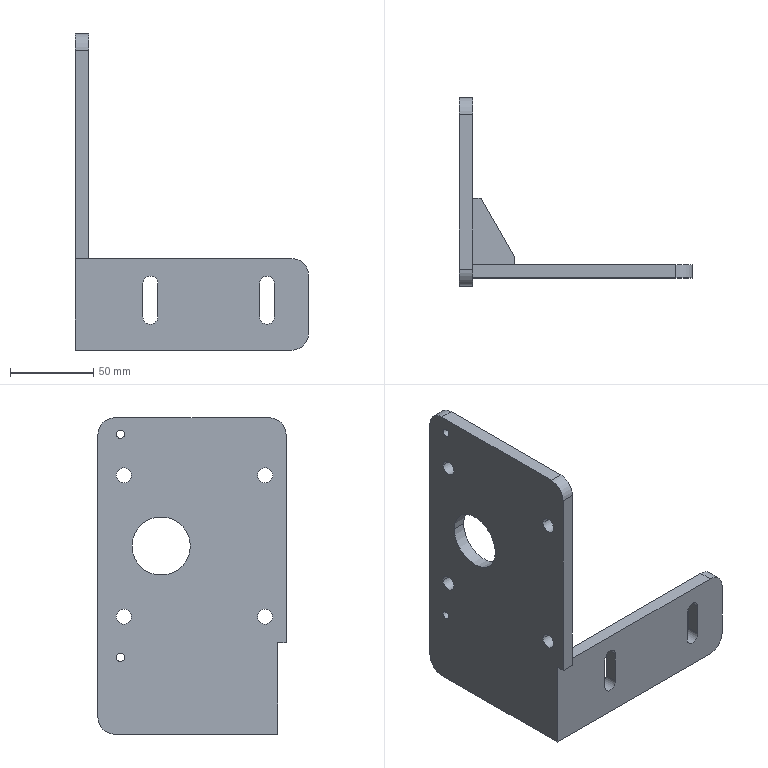Part | SolidWorks | features ICE 6, Fillet 3, Cut 1, DeleteBody 1, ExtruThin 1, MirrorSolid 1 | 2 solids | 47 faces | box 140 x 113 x 190 mm | volume 218037 mm3 | cylinder 25 | plane 22 | commonest cylinder face diameters 9 x14 20 x5 5 x4 35 x2
STEP:
#1=CARTESIAN_POINT('',(8.,48.,-95.));
#2=VERTEX_POINT('',#1);
#3=CARTESIAN_POINT('',(8.,8.,-95.));
#4=VERTEX_POINT('',#3);
#5=CARTESIAN_POINT('',(8.,8.,-95.));
#6=DIRECTION('',(0.,-1.,0.));
#7=VECTOR('',#6,1000.);
#8=LINE('',#5,#7);
#9=EDGE_CURVE('',#2,#4,#8,.T.);
#10=ORIENTED_EDGE('',*,*,#9,.T.);
#11=CARTESIAN_POINT('',(8.,8.,-87.));
#12=VERTEX_POINT('',#11);
#13=CARTESIAN_POINT('',(8.,8.,-87.));
#14=DIRECTION('',(0.,0.,-1.));
#15=VECTOR('',#14,1000.);
#16=LINE('',#13,#15);
#17=EDGE_CURVE('',#12,#4,#16,.T.);
#18=ORIENTED_EDGE('',*,*,#17,.F.);
#19=CARTESIAN_POINT('',(8.,48.,-87.));
#20=VERTEX_POINT('',#19);
#21=CARTESIAN_POINT('',(8.,8.,-87.));
#22=DIRECTION('',(0.,-1.,0.));
#23=VECTOR('',#22,1000.);
#24=LINE('',#21,#23);
#25=EDGE_CURVE('',#20,#12,#24,.T.);
#26=ORIENTED_EDGE('',*,*,#25,.F.);
#27=CARTESIAN_POINT('',(8.,48.,-87.));
#28=DIRECTION('',(0.,0.,-1.));
#29=VECTOR('',#28,1000.);
#30=LINE('',#27,#29);
#31=EDGE_CURVE('',#20,#2,#30,.T.);
#32=ORIENTED_EDGE('',*,*,#31,.T.);
#33=EDGE_LOOP('',(#10,#18,#26,#32));
#34=FACE_OUTER_BOUND('',#33,.T.);
#35=CARTESIAN_POINT('',(8.,8.,-87.));
#36=DIRECTION('',(-1.,0.,0.));
#37=DIRECTION('',(0.,0.,-1.));
#38=AXIS2_PLACEMENT_3D('',#35,#36,#37);
#39=PLANE('',#38);
#40=ADVANCED_FACE('',(#34),#39,.T.);
#41=CARTESIAN_POINT('',(13.,48.,-95.));
#42=VERTEX_POINT('',#41);
#43=CARTESIAN_POINT('',(8.,48.,-95.));
#44=DIRECTION('',(-1.,0.,0.));
#45=VECTOR('',#44,1000.);
#46=LINE('',#43,#45);
#47=EDGE_CURVE('',#42,#2,#46,.T.);
#48=ORIENTED_EDGE('',*,*,#47,.T.);
#49=ORIENTED_EDGE('',*,*,#31,.F.);
#50=CARTESIAN_POINT('',(13.,48.,-87.));
#51=VERTEX_POINT('',#50);
#52=CARTESIAN_POINT('',(8.,48.,-87.));
#53=DIRECTION('',(-1.,0.,0.));
#54=VECTOR('',#53,1000.);
#55=LINE('',#52,#54);
#56=EDGE_CURVE('',#51,#20,#55,.T.);
#57=ORIENTED_EDGE('',*,*,#56,.F.);
#58=CARTESIAN_POINT('',(13.,48.,-87.));
#59=DIRECTION('',(0.,0.,-1.));
#60=VECTOR('',#59,1000.);
#61=LINE('',#58,#60);
#62=EDGE_CURVE('',#51,#42,#61,.T.);
#63=ORIENTED_EDGE('',*,*,#62,.T.);
#64=EDGE_LOOP('',(#48,#49,#57,#63));
#65=FACE_OUTER_BOUND('',#64,.T.);
#66=CARTESIAN_POINT('',(8.,48.,-87.));
#67=DIRECTION('',(0.,1.,0.));
#68=DIRECTION('',(0.,0.,-1.));
#69=AXIS2_PLACEMENT_3D('',#66,#67,#68);
#70=PLANE('',#69);
#71=ADVANCED_FACE('',(#65),#70,.T.);
#72=CARTESIAN_POINT('',(33.,13.,-95.));
#73=VERTEX_POINT('',#72);
#74=CARTESIAN_POINT('',(13.,48.,-95.));
#75=DIRECTION('',(-0.4961,0.8682,0.));
#76=VECTOR('',#75,1000.);
#77=LINE('',#74,#76);
#78=EDGE_CURVE('',#73,#42,#77,.T.);
#79=ORIENTED_EDGE('',*,*,#78,.T.);
#80=ORIENTED_EDGE('',*,*,#62,.F.);
#81=CARTESIAN_POINT('',(33.,13.,-87.));
#82=VERTEX_POINT('',#81);
#83=CARTESIAN_POINT('',(13.,48.,-87.));
#84=DIRECTION('',(-0.4961,0.8682,0.));
#85=VECTOR('',#84,1000.);
#86=LINE('',#83,#85);
#87=EDGE_CURVE('',#82,#51,#86,.T.);
#88=ORIENTED_EDGE('',*,*,#87,.F.);
#89=CARTESIAN_POINT('',(33.,13.,-87.));
#90=DIRECTION('',(0.,0.,-1.));
#91=VECTOR('',#90,1000.);
#92=LINE('',#89,#91);
#93=EDGE_CURVE('',#82,#73,#92,.T.);
#94=ORIENTED_EDGE('',*,*,#93,.T.);
#95=EDGE_LOOP('',(#79,#80,#88,#94));
#96=FACE_OUTER_BOUND('',#95,.T.);
#97=CARTESIAN_POINT('',(13.,48.,-87.));
#98=DIRECTION('',(0.8682,0.4961,0.));
#99=DIRECTION('',(-0.4961,0.8682,0.));
#100=AXIS2_PLACEMENT_3D('',#97,#98,#99);
#101=PLANE('',#100);
#102=ADVANCED_FACE('',(#96),#101,.T.);
#103=CARTESIAN_POINT('',(33.,8.,-95.));
#104=VERTEX_POINT('',#103);
#105=CARTESIAN_POINT('',(33.,13.,-95.));
#106=DIRECTION('',(0.,1.,0.));
#107=VECTOR('',#106,1000.);
#108=LINE('',#105,#107);
#109=EDGE_CURVE('',#104,#73,#108,.T.);
#110=ORIENTED_EDGE('',*,*,#109,.T.);
#111=ORIENTED_EDGE('',*,*,#93,.F.);
#112=CARTESIAN_POINT('',(33.,8.,-87.));
#113=VERTEX_POINT('',#112);
#114=CARTESIAN_POINT('',(33.,13.,-87.));
#115=DIRECTION('',(0.,1.,0.));
#116=VECTOR('',#115,1000.);
#117=LINE('',#114,#116);
#118=EDGE_CURVE('',#113,#82,#117,.T.);
#119=ORIENTED_EDGE('',*,*,#118,.F.);
#120=CARTESIAN_POINT('',(33.,8.,-87.));
#121=DIRECTION('',(0.,0.,-1.));
#122=VECTOR('',#121,1000.);
#123=LINE('',#120,#122);
#124=EDGE_CURVE('',#113,#104,#123,.T.);
#125=ORIENTED_EDGE('',*,*,#124,.T.);
#126=EDGE_LOOP('',(#110,#111,#119,#125));
#127=FACE_OUTER_BOUND('',#126,.T.);
#128=CARTESIAN_POINT('',(33.,13.,-87.));
#129=DIRECTION('',(1.,0.,0.));
#130=DIRECTION('',(0.,0.,1.));
#131=AXIS2_PLACEMENT_3D('',#128,#129,#130);
#132=PLANE('',#131);
#133=ADVANCED_FACE('',(#127),#132,.T.);
#134=CARTESIAN_POINT('',(33.,8.,-95.));
#135=DIRECTION('',(1.,0.,0.));
#136=VECTOR('',#135,1000.);
#137=LINE('',#134,#136);
#138=EDGE_CURVE('',#4,#104,#137,.T.);
#139=ORIENTED_EDGE('',*,*,#138,.T.);
#140=ORIENTED_EDGE('',*,*,#124,.F.);
#141=CARTESIAN_POINT('',(33.,8.,-87.));
#142=DIRECTION('',(1.,0.,0.));
#143=VECTOR('',#142,1000.);
#144=LINE('',#141,#143);
#145=EDGE_CURVE('',#12,#113,#144,.T.);
#146=ORIENTED_EDGE('',*,*,#145,.F.);
#147=ORIENTED_EDGE('',*,*,#17,.T.);
#148=EDGE_LOOP('',(#139,#140,#146,#147));
#149=FACE_OUTER_BOUND('',#148,.T.);
#150=CARTESIAN_POINT('',(33.,8.,-87.));
#151=DIRECTION('',(0.,-1.,0.));
#152=DIRECTION('',(0.,0.,1.));
#153=AXIS2_PLACEMENT_3D('',#150,#151,#152);
#154=PLANE('',#153);
#155=ADVANCED_FACE('',(#149),#154,.T.);
#156=ORIENTED_EDGE('',*,*,#25,.T.);
#157=ORIENTED_EDGE('',*,*,#145,.T.);
#158=ORIENTED_EDGE('',*,*,#118,.T.);
#159=ORIENTED_EDGE('',*,*,#87,.T.);
#160=ORIENTED_EDGE('',*,*,#56,.T.);
#161=EDGE_LOOP('',(#156,#157,#158,#159,#160));
#162=FACE_OUTER_BOUND('',#161,.T.);
#163=CARTESIAN_POINT('',(0.,0.,-87.));
#164=DIRECTION('',(0.,0.,1.));
#165=DIRECTION('',(-1.,0.,0.));
#166=AXIS2_PLACEMENT_3D('',#163,#164,#165);
#167=PLANE('',#166);
#168=ADVANCED_FACE('',(#162),#167,.T.);
#169=ORIENTED_EDGE('',*,*,#9,.F.);
#170=ORIENTED_EDGE('',*,*,#47,.F.);
#171=ORIENTED_EDGE('',*,*,#78,.F.);
#172=ORIENTED_EDGE('',*,*,#109,.F.);
#173=ORIENTED_EDGE('',*,*,#138,.F.);
#174=EDGE_LOOP('',(#169,#170,#171,#172,#173));
#175=FACE_OUTER_BOUND('',#174,.T.);
#176=CARTESIAN_POINT('',(0.,0.,-95.));
#177=DIRECTION('',(0.,0.,1.));
#178=DIRECTION('',(-1.,0.,0.));
#179=AXIS2_PLACEMENT_3D('',#176,#177,#178);
#180=PLANE('',#179);
#181=ADVANCED_FACE('',(#175),#180,.F.);
#182=CLOSED_SHELL('',(#40,#71,#102,#133,#155,#168,#181));
#183=MANIFOLD_SOLID_BREP('',#182);
#184=CARTESIAN_POINT('',(0.,97.,85.142));
#185=VERTEX_POINT('',#184);
#186=CARTESIAN_POINT('',(0.,92.,85.142));
#187=VERTEX_POINT('',#186);
#188=CARTESIAN_POINT('',(0.,94.5,85.142));
#189=DIRECTION('',(-1.,0.,0.));
#190=DIRECTION('',(0.,-1.,0.));
#191=AXIS2_PLACEMENT_3D('',#188,#189,#190);
#192=CIRCLE('',#191,2.5);
#193=EDGE_CURVE('',#185,#187,#192,.T.);
#194=ORIENTED_EDGE('',*,*,#193,.T.);
#195=CARTESIAN_POINT('',(8.,92.,85.142));
#196=VERTEX_POINT('',#195);
#197=CARTESIAN_POINT('',(-2.,92.,85.142));
#198=DIRECTION('',(1.,0.,0.));
#199=VECTOR('',#198,1000.);
#200=LINE('',#197,#199);
#201=EDGE_CURVE('',#187,#196,#200,.T.);
#202=ORIENTED_EDGE('',*,*,#201,.T.);
#203=CARTESIAN_POINT('',(8.,97.,85.142));
#204=VERTEX_POINT('',#203);
#205=CARTESIAN_POINT('',(8.,94.5,85.142));
#206=DIRECTION('',(1.,0.,0.));
#207=DIRECTION('',(0.,1.,0.));
#208=AXIS2_PLACEMENT_3D('',#205,#206,#207);
#209=CIRCLE('',#208,2.5);
#210=EDGE_CURVE('',#196,#204,#209,.T.);
#211=ORIENTED_EDGE('',*,*,#210,.T.);
#212=CARTESIAN_POINT('',(-2.,97.,85.142));
#213=DIRECTION('',(1.,0.,0.));
#214=VECTOR('',#213,1000.);
#215=LINE('',#212,#214);
#216=EDGE_CURVE('',#185,#204,#215,.T.);
#217=ORIENTED_EDGE('',*,*,#216,.F.);
#218=EDGE_LOOP('',(#194,#202,#211,#217));
#219=FACE_OUTER_BOUND('',#218,.T.);
#220=CARTESIAN_POINT('',(-2.,94.5,85.142));
#221=DIRECTION('',(1.,0.,0.));
#222=DIRECTION('',(0.,1.,0.));
#223=AXIS2_PLACEMENT_3D('',#220,#221,#222);
#224=CYLINDRICAL_SURFACE('',#223,2.5);
#225=ADVANCED_FACE('',(#219),#224,.F.);
#226=CARTESIAN_POINT('',(0.,97.,-48.858));
#227=VERTEX_POINT('',#226);
#228=CARTESIAN_POINT('',(0.,92.,-48.858));
#229=VERTEX_POINT('',#228);
#230=CARTESIAN_POINT('',(0.,94.5,-48.858));
#231=DIRECTION('',(-1.,0.,0.));
#232=DIRECTION('',(0.,-1.,0.));
#233=AXIS2_PLACEMENT_3D('',#230,#231,#232);
#234=CIRCLE('',#233,2.5);
#235=EDGE_CURVE('',#227,#229,#234,.T.);
#236=ORIENTED_EDGE('',*,*,#235,.T.);
#237=CARTESIAN_POINT('',(8.,92.,-48.858));
#238=VERTEX_POINT('',#237);
#239=CARTESIAN_POINT('',(-2.,92.,-48.858));
#240=DIRECTION('',(1.,0.,0.));
#241=VECTOR('',#240,1000.);
#242=LINE('',#239,#241);
#243=EDGE_CURVE('',#229,#238,#242,.T.);
#244=ORIENTED_EDGE('',*,*,#243,.T.);
#245=CARTESIAN_POINT('',(8.,97.,-48.858));
#246=VERTEX_POINT('',#245);
#247=CARTESIAN_POINT('',(8.,94.5,-48.858));
#248=DIRECTION('',(1.,0.,0.));
#249=DIRECTION('',(0.,1.,0.));
#250=AXIS2_PLACEMENT_3D('',#247,#248,#249);
#251=CIRCLE('',#250,2.5);
#252=EDGE_CURVE('',#238,#246,#251,.T.);
#253=ORIENTED_EDGE('',*,*,#252,.T.);
#254=CARTESIAN_POINT('',(-2.,97.,-48.858));
#255=DIRECTION('',(1.,0.,0.));
#256=VECTOR('',#255,1000.);
#257=LINE('',#254,#256);
#258=EDGE_CURVE('',#227,#246,#257,.T.);
#259=ORIENTED_EDGE('',*,*,#258,.F.);
#260=EDGE_LOOP('',(#236,#244,#253,#259));
#261=FACE_OUTER_BOUND('',#260,.T.);
#262=CARTESIAN_POINT('',(-2.,94.5,-48.858));
#263=DIRECTION('',(1.,0.,0.));
#264=DIRECTION('',(0.,1.,0.));
#265=AXIS2_PLACEMENT_3D('',#262,#263,#264);
#266=CYLINDRICAL_SURFACE('',#265,2.5);
#267=ADVANCED_FACE('',(#261),#266,.F.);
#268=CARTESIAN_POINT('',(119.5,0.,-55.));
#269=VERTEX_POINT('',#268);
#270=CARTESIAN_POINT('',(115.,0.,-50.5));
#271=VERTEX_POINT('',#270);
#272=CARTESIAN_POINT('',(115.,0.,-55.));
#273=DIRECTION('',(0.,-1.,0.));
#274=DIRECTION('',(0.,0.,-1.));
#275=AXIS2_PLACEMENT_3D('',#272,#273,#274);
#276=CIRCLE('',#275,4.5);
#277=EDGE_CURVE('',#269,#271,#276,.T.);
#278=ORIENTED_EDGE('',*,*,#277,.T.);
#279=CARTESIAN_POINT('',(115.,8.,-50.5));
#280=VERTEX_POINT('',#279);
#281=CARTESIAN_POINT('',(115.,-2.,-50.5));
#282=DIRECTION('',(0.,1.,0.));
#283=VECTOR('',#282,1000.);
#284=LINE('',#281,#283);
#285=EDGE_CURVE('',#271,#280,#284,.T.);
#286=ORIENTED_EDGE('',*,*,#285,.T.);
#287=CARTESIAN_POINT('',(119.5,8.,-55.));
#288=VERTEX_POINT('',#287);
#289=CARTESIAN_POINT('',(115.,8.,-55.));
#290=DIRECTION('',(0.,1.,0.));
#291=DIRECTION('',(0.,0.,1.));
#292=AXIS2_PLACEMENT_3D('',#289,#290,#291);
#293=CIRCLE('',#292,4.5);
#294=EDGE_CURVE('',#280,#288,#293,.T.);
#295=ORIENTED_EDGE('',*,*,#294,.T.);
#296=CARTESIAN_POINT('',(119.5,-2.,-55.));
#297=DIRECTION('',(0.,1.,0.));
#298=VECTOR('',#297,1000.);
#299=LINE('',#296,#298);
#300=EDGE_CURVE('',#269,#288,#299,.T.);
#301=ORIENTED_EDGE('',*,*,#300,.F.);
#302=EDGE_LOOP('',(#278,#286,#295,#301));
#303=FACE_OUTER_BOUND('',#302,.T.);
#304=CARTESIAN_POINT('',(115.,-2.,-55.));
#305=DIRECTION('',(0.,1.,0.));
#306=DIRECTION('',(0.,0.,1.));
#307=AXIS2_PLACEMENT_3D('',#304,#305,#306);
#308=CYLINDRICAL_SURFACE('',#307,4.5);
#309=ADVANCED_FACE('',(#303),#308,.F.);
#310=CARTESIAN_POINT('',(49.5,0.,-55.));
#311=VERTEX_POINT('',#310);
#312=CARTESIAN_POINT('',(45.,0.,-50.5));
#313=VERTEX_POINT('',#312);
#314=CARTESIAN_POINT('',(45.,0.,-55.));
#315=DIRECTION('',(0.,-1.,0.));
#316=DIRECTION('',(0.,0.,-1.));
#317=AXIS2_PLACEMENT_3D('',#314,#315,#316);
#318=CIRCLE('',#317,4.5);
#319=EDGE_CURVE('',#311,#313,#318,.T.);
#320=ORIENTED_EDGE('',*,*,#319,.T.);
#321=CARTESIAN_POINT('',(45.,8.,-50.5));
#322=VERTEX_POINT('',#321);
#323=CARTESIAN_POINT('',(45.,-2.,-50.5));
#324=DIRECTION('',(0.,1.,0.));
#325=VECTOR('',#324,1000.);
#326=LINE('',#323,#325);
#327=EDGE_CURVE('',#313,#322,#326,.T.);
#328=ORIENTED_EDGE('',*,*,#327,.T.);
#329=CARTESIAN_POINT('',(49.5,8.,-55.));
#330=VERTEX_POINT('',#329);
#331=CARTESIAN_POINT('',(45.,8.,-55.));
#332=DIRECTION('',(0.,1.,0.));
#333=DIRECTION('',(0.,0.,1.));
#334=AXIS2_PLACEMENT_3D('',#331,#332,#333);
#335=CIRCLE('',#334,4.5);
#336=EDGE_CURVE('',#322,#330,#335,.T.);
#337=ORIENTED_EDGE('',*,*,#336,.T.);
#338=CARTESIAN_POINT('',(49.5,-2.,-55.));
#339=DIRECTION('',(0.,1.,0.));
#340=VECTOR('',#339,1000.);
#341=LINE('',#338,#340);
#342=EDGE_CURVE('',#311,#330,#341,.T.);
#343=ORIENTED_EDGE('',*,*,#342,.F.);
#344=EDGE_LOOP('',(#320,#328,#337,#343));
#345=FACE_OUTER_BOUND('',#344,.T.);
#346=CARTESIAN_POINT('',(45.,-2.,-55.));
#347=DIRECTION('',(0.,1.,0.));
#348=DIRECTION('',(0.,0.,1.));
#349=AXIS2_PLACEMENT_3D('',#346,#347,#348);
#350=CYLINDRICAL_SURFACE('',#349,4.5);
#351=ADVANCED_FACE('',(#345),#350,.F.);
#352=CARTESIAN_POINT('',(0.,52.5,18.));
#353=VERTEX_POINT('',#352);
#354=CARTESIAN_POINT('',(0.,87.5,18.));
#355=VERTEX_POINT('',#354);
#356=CARTESIAN_POINT('',(0.,70.,18.));
#357=DIRECTION('',(1.,0.,0.));
#358=DIRECTION('',(0.,1.,0.));
#359=AXIS2_PLACEMENT_3D('',#356,#357,#358);
#360=CIRCLE('',#359,17.5);
#361=EDGE_CURVE('',#353,#355,#360,.T.);
#362=ORIENTED_EDGE('',*,*,#361,.F.);
#363=CARTESIAN_POINT('',(8.,52.5,18.));
#364=VERTEX_POINT('',#363);
#365=CARTESIAN_POINT('',(0.,52.5,18.));
#366=DIRECTION('',(1.,0.,0.));
#367=VECTOR('',#366,1000.);
#368=LINE('',#365,#367);
#369=EDGE_CURVE('',#353,#364,#368,.T.);
#370=ORIENTED_EDGE('',*,*,#369,.T.);
#371=CARTESIAN_POINT('',(8.,87.5,18.));
#372=VERTEX_POINT('',#371);
#373=CARTESIAN_POINT('',(8.,70.,18.));
#374=DIRECTION('',(1.,0.,0.));
#375=DIRECTION('',(0.,1.,0.));
#376=AXIS2_PLACEMENT_3D('',#373,#374,#375);
#377=CIRCLE('',#376,17.5);
#378=EDGE_CURVE('',#364,#372,#377,.T.);
#379=ORIENTED_EDGE('',*,*,#378,.T.);
#380=CARTESIAN_POINT('',(0.,87.5,18.));
#381=DIRECTION('',(1.,0.,0.));
#382=VECTOR('',#381,1000.);
#383=LINE('',#380,#382);
#384=EDGE_CURVE('',#355,#372,#383,.T.);
#385=ORIENTED_EDGE('',*,*,#384,.F.);
#386=EDGE_LOOP('',(#362,#370,#379,#385));
#387=FACE_OUTER_BOUND('',#386,.T.);
#388=CARTESIAN_POINT('',(0.,70.,18.));
#389=DIRECTION('',(1.,0.,0.));
#390=DIRECTION('',(0.,1.,0.));
#391=AXIS2_PLACEMENT_3D('',#388,#389,#390);
#392=CYLINDRICAL_SURFACE('',#391,17.5);
#393=ADVANCED_FACE('',(#387),#392,.F.);
#394=CARTESIAN_POINT('',(0.,87.926,-24.426));
#395=VERTEX_POINT('',#394);
#396=CARTESIAN_POINT('',(0.,96.926,-24.426));
#397=VERTEX_POINT('',#396);
#398=CARTESIAN_POINT('',(0.,92.426,-24.426));
#399=DIRECTION('',(1.,0.,0.));
#400=DIRECTION('',(0.,1.,0.));
#401=AXIS2_PLACEMENT_3D('',#398,#399,#400);
#402=CIRCLE('',#401,4.5);
#403=EDGE_CURVE('',#395,#397,#402,.T.);
#404=ORIENTED_EDGE('',*,*,#403,.F.);
#405=CARTESIAN_POINT('',(8.,87.926,-24.426));
#406=VERTEX_POINT('',#405);
#407=CARTESIAN_POINT('',(0.,87.926,-24.426));
#408=DIRECTION('',(1.,0.,0.));
#409=VECTOR('',#408,1000.);
#410=LINE('',#407,#409);
#411=EDGE_CURVE('',#395,#406,#410,.T.);
#412=ORIENTED_EDGE('',*,*,#411,.T.);
#413=CARTESIAN_POINT('',(8.,96.926,-24.426));
#414=VERTEX_POINT('',#413);
#415=CARTESIAN_POINT('',(8.,92.426,-24.426));
#416=DIRECTION('',(1.,0.,0.));
#417=DIRECTION('',(0.,1.,0.));
#418=AXIS2_PLACEMENT_3D('',#415,#416,#417);
#419=CIRCLE('',#418,4.5);
#420=EDGE_CURVE('',#406,#414,#419,.T.);
#421=ORIENTED_EDGE('',*,*,#420,.T.);
#422=CARTESIAN_POINT('',(0.,96.926,-24.426));
#423=DIRECTION('',(1.,0.,0.));
#424=VECTOR('',#423,1000.);
#425=LINE('',#422,#424);
#426=EDGE_CURVE('',#397,#414,#425,.T.);
#427=ORIENTED_EDGE('',*,*,#426,.F.);
#428=EDGE_LOOP('',(#404,#412,#421,#427));
#429=FACE_OUTER_BOUND('',#428,.T.);
#430=CARTESIAN_POINT('',(0.,92.426,-24.426));
#431=DIRECTION('',(1.,0.,0.));
#432=DIRECTION('',(0.,1.,0.));
#433=AXIS2_PLACEMENT_3D('',#430,#431,#432);
#434=CYLINDRICAL_SURFACE('',#433,4.5);
#435=ADVANCED_FACE('',(#429),#434,.F.);
#436=CARTESIAN_POINT('',(0.,87.926,60.426));
#437=VERTEX_POINT('',#436);
#438=CARTESIAN_POINT('',(0.,96.926,60.426));
#439=VERTEX_POINT('',#438);
#440=CARTESIAN_POINT('',(0.,92.426,60.426));
#441=DIRECTION('',(1.,0.,0.));
#442=DIRECTION('',(0.,1.,0.));
#443=AXIS2_PLACEMENT_3D('',#440,#441,#442);
#444=CIRCLE('',#443,4.5);
#445=EDGE_CURVE('',#437,#439,#444,.T.);
#446=ORIENTED_EDGE('',*,*,#445,.F.);
#447=CARTESIAN_POINT('',(8.,87.926,60.426));
#448=VERTEX_POINT('',#447);
#449=CARTESIAN_POINT('',(0.,87.926,60.426));
#450=DIRECTION('',(1.,0.,0.));
#451=VECTOR('',#450,1000.);
#452=LINE('',#449,#451);
#453=EDGE_CURVE('',#437,#448,#452,.T.);
#454=ORIENTED_EDGE('',*,*,#453,.T.);
#455=CARTESIAN_POINT('',(8.,96.926,60.426));
#456=VERTEX_POINT('',#455);
#457=CARTESIAN_POINT('',(8.,92.426,60.426));
#458=DIRECTION('',(1.,0.,0.));
#459=DIRECTION('',(0.,1.,0.));
#460=AXIS2_PLACEMENT_3D('',#457,#458,#459);
#461=CIRCLE('',#460,4.5);
#462=EDGE_CURVE('',#448,#456,#461,.T.);
#463=ORIENTED_EDGE('',*,*,#462,.T.);
#464=CARTESIAN_POINT('',(0.,96.926,60.426));
#465=DIRECTION('',(1.,0.,0.));
#466=VECTOR('',#465,1000.);
#467=LINE('',#464,#466);
#468=EDGE_CURVE('',#439,#456,#467,.T.);
#469=ORIENTED_EDGE('',*,*,#468,.F.);
#470=EDGE_LOOP('',(#446,#454,#463,#469));
#471=FACE_OUTER_BOUND('',#470,.T.);
#472=CARTESIAN_POINT('',(0.,92.426,60.426));
#473=DIRECTION('',(1.,0.,0.));
#474=DIRECTION('',(0.,1.,0.));
#475=AXIS2_PLACEMENT_3D('',#472,#473,#474);
#476=CYLINDRICAL_SURFACE('',#475,4.5);
#477=ADVANCED_FACE('',(#471),#476,.F.);
#478=CARTESIAN_POINT('',(0.,3.074,-24.426));
#479=VERTEX_POINT('',#478);
#480=CARTESIAN_POINT('',(0.,12.074,-24.426));
#481=VERTEX_POINT('',#480);
#482=CARTESIAN_POINT('',(0.,7.574,-24.426));
#483=DIRECTION('',(1.,0.,0.));
#484=DIRECTION('',(0.,1.,0.));
#485=AXIS2_PLACEMENT_3D('',#482,#483,#484);
#486=CIRCLE('',#485,4.5);
#487=EDGE_CURVE('',#479,#481,#486,.T.);
#488=ORIENTED_EDGE('',*,*,#487,.F.);
#489=CARTESIAN_POINT('',(8.,3.074,-24.426));
#490=VERTEX_POINT('',#489);
#491=CARTESIAN_POINT('',(0.,3.074,-24.426));
#492=DIRECTION('',(1.,0.,0.));
#493=VECTOR('',#492,1000.);
#494=LINE('',#491,#493);
#495=EDGE_CURVE('',#479,#490,#494,.T.);
#496=ORIENTED_EDGE('',*,*,#495,.T.);
#497=CARTESIAN_POINT('',(8.,12.074,-24.426));
#498=VERTEX_POINT('',#497);
#499=CARTESIAN_POINT('',(8.,7.574,-24.426));
#500=DIRECTION('',(1.,0.,0.));
#501=DIRECTION('',(0.,1.,0.));
#502=AXIS2_PLACEMENT_3D('',#499,#500,#501);
#503=CIRCLE('',#502,4.5);
#504=EDGE_CURVE('',#490,#498,#503,.T.);
#505=ORIENTED_EDGE('',*,*,#504,.T.);
#506=CARTESIAN_POINT('',(0.,12.074,-24.426));
#507=DIRECTION('',(1.,0.,0.));
#508=VECTOR('',#507,1000.);
#509=LINE('',#506,#508);
#510=EDGE_CURVE('',#481,#498,#509,.T.);
#511=ORIENTED_EDGE('',*,*,#510,.F.);
#512=EDGE_LOOP('',(#488,#496,#505,#511));
#513=FACE_OUTER_BOUND('',#512,.T.);
#514=CARTESIAN_POINT('',(0.,7.574,-24.426));
#515=DIRECTION('',(1.,0.,0.));
#516=DIRECTION('',(0.,1.,0.));
#517=AXIS2_PLACEMENT_3D('',#514,#515,#516);
#518=CYLINDRICAL_SURFACE('',#517,4.5);
#519=ADVANCED_FACE('',(#513),#518,.F.);
#520=CARTESIAN_POINT('',(0.,3.074,60.426));
#521=VERTEX_POINT('',#520);
#522=CARTESIAN_POINT('',(0.,12.074,60.426));
#523=VERTEX_POINT('',#522);
#524=CARTESIAN_POINT('',(0.,7.574,60.426));
#525=DIRECTION('',(1.,0.,0.));
#526=DIRECTION('',(0.,1.,0.));
#527=AXIS2_PLACEMENT_3D('',#524,#525,#526);
#528=CIRCLE('',#527,4.5);
#529=EDGE_CURVE('',#521,#523,#528,.T.);
#530=ORIENTED_EDGE('',*,*,#529,.F.);
#531=CARTESIAN_POINT('',(8.,3.074,60.426));
#532=VERTEX_POINT('',#531);
#533=CARTESIAN_POINT('',(0.,3.074,60.426));
#534=DIRECTION('',(1.,0.,0.));
#535=VECTOR('',#534,1000.);
#536=LINE('',#533,#535);
#537=EDGE_CURVE('',#521,#532,#536,.T.);
#538=ORIENTED_EDGE('',*,*,#537,.T.);
#539=CARTESIAN_POINT('',(8.,12.074,60.426));
#540=VERTEX_POINT('',#539);
#541=CARTESIAN_POINT('',(8.,7.574,60.426));
#542=DIRECTION('',(1.,0.,0.));
#543=DIRECTION('',(0.,1.,0.));
#544=AXIS2_PLACEMENT_3D('',#541,#542,#543);
#545=CIRCLE('',#544,4.5);
#546=EDGE_CURVE('',#532,#540,#545,.T.);
#547=ORIENTED_EDGE('',*,*,#546,.T.);
#548=CARTESIAN_POINT('',(0.,12.074,60.426));
#549=DIRECTION('',(1.,0.,0.));
#550=VECTOR('',#549,1000.);
#551=LINE('',#548,#550);
#552=EDGE_CURVE('',#523,#540,#551,.T.);
#553=ORIENTED_EDGE('',*,*,#552,.F.);
#554=EDGE_LOOP('',(#530,#538,#547,#553));
#555=FACE_OUTER_BOUND('',#554,.T.);
#556=CARTESIAN_POINT('',(0.,7.574,60.426));
#557=DIRECTION('',(1.,0.,0.));
#558=DIRECTION('',(0.,1.,0.));
#559=AXIS2_PLACEMENT_3D('',#556,#557,#558);
#560=CYLINDRICAL_SURFACE('',#559,4.5);
#561=ADVANCED_FACE('',(#555),#560,.F.);
#562=CARTESIAN_POINT('',(0.,0.,-40.));
#563=VERTEX_POINT('',#562);
#564=CARTESIAN_POINT('',(8.,0.,-40.));
#565=VERTEX_POINT('',#564);
#566=CARTESIAN_POINT('',(8.,0.,-40.));
#567=DIRECTION('',(1.,0.,0.));
#568=VECTOR('',#567,1000.);
#569=LINE('',#566,#568);
#570=EDGE_CURVE('',#563,#565,#569,.T.);
#571=ORIENTED_EDGE('',*,*,#570,.F.);
#572=CARTESIAN_POINT('',(0.,0.,-95.));
#573=VERTEX_POINT('',#572);
#574=CARTESIAN_POINT('',(0.,0.,-95.));
#575=DIRECTION('',(0.,0.,1.));
#576=VECTOR('',#575,1000.);
#577=LINE('',#574,#576);
#578=EDGE_CURVE('',#573,#563,#577,.T.);
#579=ORIENTED_EDGE('',*,*,#578,.F.);
#580=CARTESIAN_POINT('',(130.,0.,-95.));
#581=VERTEX_POINT('',#580);
#582=CARTESIAN_POINT('',(0.,0.,-95.));
#583=DIRECTION('',(1.,0.,0.));
#584=VECTOR('',#583,1000.);
#585=LINE('',#582,#584);
#586=EDGE_CURVE('',#573,#581,#585,.T.);
#587=ORIENTED_EDGE('',*,*,#586,.T.);
#588=CARTESIAN_POINT('',(140.,0.,-85.));
#589=VERTEX_POINT('',#588);
#590=CARTESIAN_POINT('',(130.,0.,-85.));
#591=DIRECTION('',(0.,-1.,0.));
#592=DIRECTION('',(0.,0.,-1.));
#593=AXIS2_PLACEMENT_3D('',#590,#591,#592);
#594=CIRCLE('',#593,10.);
#595=EDGE_CURVE('',#581,#589,#594,.T.);
#596=ORIENTED_EDGE('',*,*,#595,.T.);
#597=CARTESIAN_POINT('',(140.,0.,-50.));
#598=VERTEX_POINT('',#597);
#599=CARTESIAN_POINT('',(140.,0.,-95.));
#600=DIRECTION('',(0.,0.,1.));
#601=VECTOR('',#600,1000.);
#602=LINE('',#599,#601);
#603=EDGE_CURVE('',#589,#598,#602,.T.);
#604=ORIENTED_EDGE('',*,*,#603,.T.);
#605=CARTESIAN_POINT('',(130.,0.,-40.));
#606=VERTEX_POINT('',#605);
#607=CARTESIAN_POINT('',(130.,0.,-50.));
#608=DIRECTION('',(0.,-1.,0.));
#609=DIRECTION('',(0.,0.,-1.));
#610=AXIS2_PLACEMENT_3D('',#607,#608,#609);
#611=CIRCLE('',#610,10.);
#612=EDGE_CURVE('',#598,#606,#611,.T.);
#613=ORIENTED_EDGE('',*,*,#612,.T.);
#614=CARTESIAN_POINT('',(0.,0.,-40.));
#615=DIRECTION('',(1.,0.,0.));
#616=VECTOR('',#615,1000.);
#617=LINE('',#614,#616);
#618=EDGE_CURVE('',#565,#606,#617,.T.);
#619=ORIENTED_EDGE('',*,*,#618,.F.);
#620=EDGE_LOOP('',(#571,#579,#587,#596,#604,#613,#619));
#621=FACE_OUTER_BOUND('',#620,.T.);
#622=ORIENTED_EDGE('',*,*,#277,.F.);
#623=CARTESIAN_POINT('',(119.5,0.,-75.));
#624=VERTEX_POINT('',#623);
#625=CARTESIAN_POINT('',(119.5,0.,-95.));
#626=DIRECTION('',(0.,0.,1.));
#627=VECTOR('',#626,1000.);
#628=LINE('',#625,#627);
#629=EDGE_CURVE('',#624,#269,#628,.T.);
#630=ORIENTED_EDGE('',*,*,#629,.F.);
#631=CARTESIAN_POINT('',(110.5,0.,-75.));
#632=VERTEX_POINT('',#631);
#633=CARTESIAN_POINT('',(115.,0.,-75.));
#634=DIRECTION('',(0.,-1.,0.));
#635=DIRECTION('',(0.,0.,-1.));
#636=AXIS2_PLACEMENT_3D('',#633,#634,#635);
#637=CIRCLE('',#636,4.5);
#638=EDGE_CURVE('',#632,#624,#637,.T.);
#639=ORIENTED_EDGE('',*,*,#638,.F.);
#640=CARTESIAN_POINT('',(110.5,0.,-55.));
#641=VERTEX_POINT('',#640);
#642=CARTESIAN_POINT('',(110.5,0.,-95.));
#643=DIRECTION('',(0.,0.,-1.));
#644=VECTOR('',#643,1000.);
#645=LINE('',#642,#644);
#646=EDGE_CURVE('',#641,#632,#645,.T.);
#647=ORIENTED_EDGE('',*,*,#646,.F.);
#648=CARTESIAN_POINT('',(115.,0.,-55.));
#649=DIRECTION('',(0.,-1.,0.));
#650=DIRECTION('',(0.,0.,-1.));
#651=AXIS2_PLACEMENT_3D('',#648,#649,#650);
#652=CIRCLE('',#651,4.5);
#653=EDGE_CURVE('',#271,#641,#652,.T.);
#654=ORIENTED_EDGE('',*,*,#653,.F.);
#655=EDGE_LOOP('',(#622,#630,#639,#647,#654));
#656=FACE_BOUND('',#655,.T.);
#657=ORIENTED_EDGE('',*,*,#319,.F.);
#658=CARTESIAN_POINT('',(49.5,0.,-75.));
#659=VERTEX_POINT('',#658);
#660=CARTESIAN_POINT('',(49.5,0.,-95.));
#661=DIRECTION('',(0.,0.,1.));
#662=VECTOR('',#661,1000.);
#663=LINE('',#660,#662);
#664=EDGE_CURVE('',#659,#311,#663,.T.);
#665=ORIENTED_EDGE('',*,*,#664,.F.);
#666=CARTESIAN_POINT('',(40.5,0.,-75.));
#667=VERTEX_POINT('',#666);
#668=CARTESIAN_POINT('',(45.,0.,-75.));
#669=DIRECTION('',(0.,-1.,0.));
#670=DIRECTION('',(0.,0.,-1.));
#671=AXIS2_PLACEMENT_3D('',#668,#669,#670);
#672=CIRCLE('',#671,4.5);
#673=EDGE_CURVE('',#667,#659,#672,.T.);
#674=ORIENTED_EDGE('',*,*,#673,.F.);
#675=CARTESIAN_POINT('',(40.5,0.,-55.));
#676=VERTEX_POINT('',#675);
#677=CARTESIAN_POINT('',(40.5,0.,-95.));
#678=DIRECTION('',(0.,0.,-1.));
#679=VECTOR('',#678,1000.);
#680=LINE('',#677,#679);
#681=EDGE_CURVE('',#676,#667,#680,.T.);
#682=ORIENTED_EDGE('',*,*,#681,.F.);
#683=CARTESIAN_POINT('',(45.,0.,-55.));
#684=DIRECTION('',(0.,-1.,0.));
#685=DIRECTION('',(0.,0.,-1.));
#686=AXIS2_PLACEMENT_3D('',#683,#684,#685);
#687=CIRCLE('',#686,4.5);
#688=EDGE_CURVE('',#313,#676,#687,.T.);
#689=ORIENTED_EDGE('',*,*,#688,.F.);
#690=EDGE_LOOP('',(#657,#665,#674,#682,#689));
#691=FACE_BOUND('',#690,.T.);
#692=CARTESIAN_POINT('',(0.,0.,-95.));
#693=DIRECTION('',(0.,-1.,0.));
#694=DIRECTION('',(0.,0.,-1.));
#695=AXIS2_PLACEMENT_3D('',#692,#693,#694);
#696=PLANE('',#695);
#697=ADVANCED_FACE('',(#621,#656,#691),#696,.T.);
#698=ORIENTED_EDGE('',*,*,#193,.F.);
#699=CARTESIAN_POINT('',(0.,94.5,85.142));
#700=DIRECTION('',(-1.,0.,0.));
#701=DIRECTION('',(0.,-1.,0.));
#702=AXIS2_PLACEMENT_3D('',#699,#700,#701);
#703=CIRCLE('',#702,2.5);
#704=EDGE_CURVE('',#187,#185,#703,.T.);
#705=ORIENTED_EDGE('',*,*,#704,.F.);
#706=EDGE_LOOP('',(#698,#705));
#707=FACE_BOUND('',#706,.T.);
#708=ORIENTED_EDGE('',*,*,#235,.F.);
#709=CARTESIAN_POINT('',(0.,94.5,-48.858));
#710=DIRECTION('',(-1.,0.,0.));
#711=DIRECTION('',(0.,-1.,0.));
#712=AXIS2_PLACEMENT_3D('',#709,#710,#711);
#713=CIRCLE('',#712,2.5);
#714=EDGE_CURVE('',#229,#227,#713,.T.);
#715=ORIENTED_EDGE('',*,*,#714,.F.);
#716=EDGE_LOOP('',(#708,#715));
#717=FACE_BOUND('',#716,.T.);
#718=CARTESIAN_POINT('',(0.,70.,18.));
#719=DIRECTION('',(1.,0.,0.));
#720=DIRECTION('',(0.,1.,0.));
#721=AXIS2_PLACEMENT_3D('',#718,#719,#720);
#722=CIRCLE('',#721,17.5);
#723=EDGE_CURVE('',#355,#353,#722,.T.);
#724=ORIENTED_EDGE('',*,*,#723,.T.);
#725=ORIENTED_EDGE('',*,*,#361,.T.);
#726=EDGE_LOOP('',(#724,#725));
#727=FACE_BOUND('',#726,.T.);
#728=CARTESIAN_POINT('',(0.,92.426,-24.426));
#729=DIRECTION('',(1.,0.,0.));
#730=DIRECTION('',(0.,1.,0.));
#731=AXIS2_PLACEMENT_3D('',#728,#729,#730);
#732=CIRCLE('',#731,4.5);
#733=EDGE_CURVE('',#397,#395,#732,.T.);
#734=ORIENTED_EDGE('',*,*,#733,.T.);
#735=ORIENTED_EDGE('',*,*,#403,.T.);
#736=EDGE_LOOP('',(#734,#735));
#737=FACE_BOUND('',#736,.T.);
#738=CARTESIAN_POINT('',(0.,7.574,-24.426));
#739=DIRECTION('',(1.,0.,0.));
#740=DIRECTION('',(0.,1.,0.));
#741=AXIS2_PLACEMENT_3D('',#738,#739,#740);
#742=CIRCLE('',#741,4.5);
#743=EDGE_CURVE('',#481,#479,#742,.T.);
#744=ORIENTED_EDGE('',*,*,#743,.T.);
#745=ORIENTED_EDGE('',*,*,#487,.T.);
#746=EDGE_LOOP('',(#744,#745));
#747=FACE_BOUND('',#746,.T.);
#748=CARTESIAN_POINT('',(0.,7.574,60.426));
#749=DIRECTION('',(1.,0.,0.));
#750=DIRECTION('',(0.,1.,0.));
#751=AXIS2_PLACEMENT_3D('',#748,#749,#750);
#752=CIRCLE('',#751,4.5);
#753=EDGE_CURVE('',#523,#521,#752,.T.);
#754=ORIENTED_EDGE('',*,*,#753,.T.);
#755=ORIENTED_EDGE('',*,*,#529,.T.);
#756=EDGE_LOOP('',(#754,#755));
#757=FACE_BOUND('',#756,.T.);
#758=CARTESIAN_POINT('',(0.,92.426,60.426));
#759=DIRECTION('',(1.,0.,0.));
#760=DIRECTION('',(0.,1.,0.));
#761=AXIS2_PLACEMENT_3D('',#758,#759,#760);
#762=CIRCLE('',#761,4.5);
#763=EDGE_CURVE('',#439,#437,#762,.T.);
#764=ORIENTED_EDGE('',*,*,#763,.T.);
#765=ORIENTED_EDGE('',*,*,#445,.T.);
#766=EDGE_LOOP('',(#764,#765));
#767=FACE_BOUND('',#766,.T.);
#768=CARTESIAN_POINT('',(0.,-5.,85.));
#769=VERTEX_POINT('',#768);
#770=CARTESIAN_POINT('',(0.,-5.,-40.));
#771=VERTEX_POINT('',#770);
#772=CARTESIAN_POINT('',(0.,-5.,-40.));
#773=DIRECTION('',(0.,0.,-1.));
#774=VECTOR('',#773,1000.);
#775=LINE('',#772,#774);
#776=EDGE_CURVE('',#769,#771,#775,.T.);
#777=ORIENTED_EDGE('',*,*,#776,.F.);
#778=CARTESIAN_POINT('',(0.,5.,95.));
#779=VERTEX_POINT('',#778);
#780=CARTESIAN_POINT('',(0.,5.,85.));
#781=DIRECTION('',(-1.,0.,0.));
#782=DIRECTION('',(0.,-1.,0.));
#783=AXIS2_PLACEMENT_3D('',#780,#781,#782);
#784=CIRCLE('',#783,10.);
#785=EDGE_CURVE('',#769,#779,#784,.T.);
#786=ORIENTED_EDGE('',*,*,#785,.T.);
#787=CARTESIAN_POINT('',(0.,98.,95.));
#788=VERTEX_POINT('',#787);
#789=CARTESIAN_POINT('',(0.,108.,95.));
#790=DIRECTION('',(0.,-1.,0.));
#791=VECTOR('',#790,1000.);
#792=LINE('',#789,#791);
#793=EDGE_CURVE('',#788,#779,#792,.T.);
#794=ORIENTED_EDGE('',*,*,#793,.F.);
#795=CARTESIAN_POINT('',(0.,108.,85.));
#796=VERTEX_POINT('',#795);
#797=CARTESIAN_POINT('',(0.,98.,85.));
#798=DIRECTION('',(-1.,0.,0.));
#799=DIRECTION('',(0.,-1.,0.));
#800=AXIS2_PLACEMENT_3D('',#797,#798,#799);
#801=CIRCLE('',#800,10.);
#802=EDGE_CURVE('',#788,#796,#801,.T.);
#803=ORIENTED_EDGE('',*,*,#802,.T.);
#804=CARTESIAN_POINT('',(0.,108.,-85.));
#805=VERTEX_POINT('',#804);
#806=CARTESIAN_POINT('',(0.,108.,-95.));
#807=DIRECTION('',(0.,0.,1.));
#808=VECTOR('',#807,1000.);
#809=LINE('',#806,#808);
#810=EDGE_CURVE('',#805,#796,#809,.T.);
#811=ORIENTED_EDGE('',*,*,#810,.F.);
#812=CARTESIAN_POINT('',(0.,98.,-95.));
#813=VERTEX_POINT('',#812);
#814=CARTESIAN_POINT('',(0.,98.,-85.));
#815=DIRECTION('',(-1.,0.,0.));
#816=DIRECTION('',(0.,-1.,0.));
#817=AXIS2_PLACEMENT_3D('',#814,#815,#816);
#818=CIRCLE('',#817,10.);
#819=EDGE_CURVE('',#805,#813,#818,.T.);
#820=ORIENTED_EDGE('',*,*,#819,.T.);
#821=CARTESIAN_POINT('',(0.,108.,-95.));
#822=DIRECTION('',(0.,-1.,0.));
#823=VECTOR('',#822,1000.);
#824=LINE('',#821,#823);
#825=EDGE_CURVE('',#813,#573,#824,.T.);
#826=ORIENTED_EDGE('',*,*,#825,.T.);
#827=ORIENTED_EDGE('',*,*,#578,.T.);
#828=CARTESIAN_POINT('',(0.,-5.,-40.));
#829=DIRECTION('',(0.,1.,0.));
#830=VECTOR('',#829,1000.);
#831=LINE('',#828,#830);
#832=EDGE_CURVE('',#771,#563,#831,.T.);
#833=ORIENTED_EDGE('',*,*,#832,.F.);
#834=EDGE_LOOP('',(#777,#786,#794,#803,#811,#820,#826,#827,#833));
#835=FACE_OUTER_BOUND('',#834,.T.);
#836=CARTESIAN_POINT('',(0.,108.,-95.));
#837=DIRECTION('',(-1.,0.,0.));
#838=DIRECTION('',(0.,-1.,0.));
#839=AXIS2_PLACEMENT_3D('',#836,#837,#838);
#840=PLANE('',#839);
#841=ADVANCED_FACE('',(#707,#717,#727,#737,#747,#757,#767,#835),#840,.T.);
#842=CARTESIAN_POINT('',(8.,108.,-85.));
#843=VERTEX_POINT('',#842);
#844=CARTESIAN_POINT('',(8.,108.,85.));
#845=VERTEX_POINT('',#844);
#846=CARTESIAN_POINT('',(8.,108.,-95.));
#847=DIRECTION('',(0.,0.,1.));
#848=VECTOR('',#847,1000.);
#849=LINE('',#846,#848);
#850=EDGE_CURVE('',#843,#845,#849,.T.);
#851=ORIENTED_EDGE('',*,*,#850,.F.);
#852=CARTESIAN_POINT('',(0.,108.,-85.));
#853=DIRECTION('',(-1.,0.,0.));
#854=VECTOR('',#853,1000.);
#855=LINE('',#852,#854);
#856=EDGE_CURVE('',#843,#805,#855,.T.);
#857=ORIENTED_EDGE('',*,*,#856,.T.);
#858=ORIENTED_EDGE('',*,*,#810,.T.);
#859=CARTESIAN_POINT('',(0.,108.,85.));
#860=DIRECTION('',(1.,0.,0.));
#861=VECTOR('',#860,1000.);
#862=LINE('',#859,#861);
#863=EDGE_CURVE('',#796,#845,#862,.T.);
#864=ORIENTED_EDGE('',*,*,#863,.T.);
#865=EDGE_LOOP('',(#851,#857,#858,#864));
#866=FACE_OUTER_BOUND('',#865,.T.);
#867=CARTESIAN_POINT('',(0.,108.,-95.));
#868=DIRECTION('',(0.,-1.,0.));
#869=DIRECTION('',(0.,0.,-1.));
#870=AXIS2_PLACEMENT_3D('',#867,#868,#869);
#871=PLANE('',#870);
#872=ADVANCED_FACE('',(#866),#871,.F.);
#873=CARTESIAN_POINT('',(8.,94.5,85.142));
#874=DIRECTION('',(1.,0.,0.));
#875=DIRECTION('',(0.,1.,0.));
#876=AXIS2_PLACEMENT_3D('',#873,#874,#875);
#877=CIRCLE('',#876,2.5);
#878=EDGE_CURVE('',#204,#196,#877,.T.);
#879=ORIENTED_EDGE('',*,*,#878,.F.);
#880=ORIENTED_EDGE('',*,*,#210,.F.);
#881=EDGE_LOOP('',(#879,#880));
#882=FACE_BOUND('',#881,.T.);
#883=CARTESIAN_POINT('',(8.,94.5,-48.858));
#884=DIRECTION('',(1.,0.,0.));
#885=DIRECTION('',(0.,1.,0.));
#886=AXIS2_PLACEMENT_3D('',#883,#884,#885);
#887=CIRCLE('',#886,2.5);
#888=EDGE_CURVE('',#246,#238,#887,.T.);
#889=ORIENTED_EDGE('',*,*,#888,.F.);
#890=ORIENTED_EDGE('',*,*,#252,.F.);
#891=EDGE_LOOP('',(#889,#890));
#892=FACE_BOUND('',#891,.T.);
#893=CARTESIAN_POINT('',(8.,98.,95.));
#894=VERTEX_POINT('',#893);
#895=CARTESIAN_POINT('',(8.,5.,95.));
#896=VERTEX_POINT('',#895);
#897=CARTESIAN_POINT('',(8.,108.,95.));
#898=DIRECTION('',(0.,-1.,0.));
#899=VECTOR('',#898,1000.);
#900=LINE('',#897,#899);
#901=EDGE_CURVE('',#894,#896,#900,.T.);
#902=ORIENTED_EDGE('',*,*,#901,.T.);
#903=CARTESIAN_POINT('',(8.,-5.,85.));
#904=VERTEX_POINT('',#903);
#905=CARTESIAN_POINT('',(8.,5.,85.));
#906=DIRECTION('',(1.,0.,0.));
#907=DIRECTION('',(0.,-1.,0.));
#908=AXIS2_PLACEMENT_3D('',#905,#906,#907);
#909=CIRCLE('',#908,10.);
#910=EDGE_CURVE('',#896,#904,#909,.T.);
#911=ORIENTED_EDGE('',*,*,#910,.T.);
#912=CARTESIAN_POINT('',(8.,-5.,-40.));
#913=VERTEX_POINT('',#912);
#914=CARTESIAN_POINT('',(8.,-5.,-40.));
#915=DIRECTION('',(0.,0.,1.));
#916=VECTOR('',#915,1000.);
#917=LINE('',#914,#916);
#918=EDGE_CURVE('',#913,#904,#917,.T.);
#919=ORIENTED_EDGE('',*,*,#918,.F.);
#920=CARTESIAN_POINT('',(8.,-5.,-40.));
#921=DIRECTION('',(0.,1.,0.));
#922=VECTOR('',#921,1000.);
#923=LINE('',#920,#922);
#924=EDGE_CURVE('',#913,#565,#923,.T.);
#925=ORIENTED_EDGE('',*,*,#924,.T.);
#926=CARTESIAN_POINT('',(8.,8.,-40.));
#927=VERTEX_POINT('',#926);
#928=CARTESIAN_POINT('',(8.,-2.,-40.));
#929=DIRECTION('',(0.,1.,0.));
#930=VECTOR('',#929,1000.);
#931=LINE('',#928,#930);
#932=EDGE_CURVE('',#565,#927,#931,.T.);
#933=ORIENTED_EDGE('',*,*,#932,.T.);
#934=CARTESIAN_POINT('',(8.,8.,-95.));
#935=VERTEX_POINT('',#934);
#936=CARTESIAN_POINT('',(8.,8.,-95.));
#937=DIRECTION('',(0.,0.,1.));
#938=VECTOR('',#937,1000.);
#939=LINE('',#936,#938);
#940=EDGE_CURVE('',#935,#927,#939,.T.);
#941=ORIENTED_EDGE('',*,*,#940,.F.);
#942=CARTESIAN_POINT('',(8.,98.,-95.));
#943=VERTEX_POINT('',#942);
#944=CARTESIAN_POINT('',(8.,108.,-95.));
#945=DIRECTION('',(0.,-1.,0.));
#946=VECTOR('',#945,1000.);
#947=LINE('',#944,#946);
#948=EDGE_CURVE('',#943,#935,#947,.T.);
#949=ORIENTED_EDGE('',*,*,#948,.F.);
#950=CARTESIAN_POINT('',(8.,98.,-85.));
#951=DIRECTION('',(1.,0.,0.));
#952=DIRECTION('',(0.,-1.,0.));
#953=AXIS2_PLACEMENT_3D('',#950,#951,#952);
#954=CIRCLE('',#953,10.);
#955=EDGE_CURVE('',#943,#843,#954,.T.);
#956=ORIENTED_EDGE('',*,*,#955,.T.);
#957=ORIENTED_EDGE('',*,*,#850,.T.);
#958=CARTESIAN_POINT('',(8.,98.,85.));
#959=DIRECTION('',(1.,0.,0.));
#960=DIRECTION('',(0.,-1.,0.));
#961=AXIS2_PLACEMENT_3D('',#958,#959,#960);
#962=CIRCLE('',#961,10.);
#963=EDGE_CURVE('',#845,#894,#962,.T.);
#964=ORIENTED_EDGE('',*,*,#963,.T.);
#965=EDGE_LOOP('',(#902,#911,#919,#925,#933,#941,#949,#956,#957,#964));
#966=FACE_OUTER_BOUND('',#965,.T.);
#967=CARTESIAN_POINT('',(8.,7.574,60.426));
#968=DIRECTION('',(1.,0.,0.));
#969=DIRECTION('',(0.,1.,0.));
#970=AXIS2_PLACEMENT_3D('',#967,#968,#969);
#971=CIRCLE('',#970,4.5);
#972=EDGE_CURVE('',#540,#532,#971,.T.);
#973=ORIENTED_EDGE('',*,*,#972,.F.);
#974=ORIENTED_EDGE('',*,*,#546,.F.);
#975=EDGE_LOOP('',(#973,#974));
#976=FACE_BOUND('',#975,.T.);
#977=CARTESIAN_POINT('',(8.,70.,18.));
#978=DIRECTION('',(1.,0.,0.));
#979=DIRECTION('',(0.,1.,0.));
#980=AXIS2_PLACEMENT_3D('',#977,#978,#979);
#981=CIRCLE('',#980,17.5);
#982=EDGE_CURVE('',#372,#364,#981,.T.);
#983=ORIENTED_EDGE('',*,*,#982,.F.);
#984=ORIENTED_EDGE('',*,*,#378,.F.);
#985=EDGE_LOOP('',(#983,#984));
#986=FACE_BOUND('',#985,.T.);
#987=CARTESIAN_POINT('',(8.,92.426,-24.426));
#988=DIRECTION('',(1.,0.,0.));
#989=DIRECTION('',(0.,1.,0.));
#990=AXIS2_PLACEMENT_3D('',#987,#988,#989);
#991=CIRCLE('',#990,4.5);
#992=EDGE_CURVE('',#414,#406,#991,.T.);
#993=ORIENTED_EDGE('',*,*,#992,.F.);
#994=ORIENTED_EDGE('',*,*,#420,.F.);
#995=EDGE_LOOP('',(#993,#994));
#996=FACE_BOUND('',#995,.T.);
#997=CARTESIAN_POINT('',(8.,92.426,60.426));
#998=DIRECTION('',(1.,0.,0.));
#999=DIRECTION('',(0.,1.,0.));
#1000=AXIS2_PLACEMENT_3D('',#997,#998,#999);
#1001=CIRCLE('',#1000,4.5);
#1002=EDGE_CURVE('',#456,#448,#1001,.T.);
#1003=ORIENTED_EDGE('',*,*,#1002,.F.);
#1004=ORIENTED_EDGE('',*,*,#462,.F.);
#1005=EDGE_LOOP('',(#1003,#1004));
#1006=FACE_BOUND('',#1005,.T.);
#1007=CARTESIAN_POINT('',(8.,7.574,-24.426));
#1008=DIRECTION('',(1.,0.,0.));
#1009=DIRECTION('',(0.,1.,0.));
#1010=AXIS2_PLACEMENT_3D('',#1007,#1008,#1009);
#1011=CIRCLE('',#1010,4.5);
#1012=EDGE_CURVE('',#498,#490,#1011,.T.);
#1013=ORIENTED_EDGE('',*,*,#1012,.F.);
#1014=ORIENTED_EDGE('',*,*,#504,.F.);
#1015=EDGE_LOOP('',(#1013,#1014));
#1016=FACE_BOUND('',#1015,.T.);
#1017=CARTESIAN_POINT('',(8.,108.,-95.));
#1018=DIRECTION('',(-1.,0.,0.));
#1019=DIRECTION('',(0.,-1.,0.));
#1020=AXIS2_PLACEMENT_3D('',#1017,#1018,#1019);
#1021=PLANE('',#1020);
#1022=ADVANCED_FACE('',(#882,#892,#966,#976,#986,#996,#1006,#1016),#1021,.F.);
#1023=CARTESIAN_POINT('',(49.5,8.,-75.));
#1024=VERTEX_POINT('',#1023);
#1025=CARTESIAN_POINT('',(49.5,8.,-55.));
#1026=DIRECTION('',(0.,0.,-1.));
#1027=VECTOR('',#1026,1000.);
#1028=LINE('',#1025,#1027);
#1029=EDGE_CURVE('',#330,#1024,#1028,.T.);
#1030=ORIENTED_EDGE('',*,*,#1029,.F.);
#1031=ORIENTED_EDGE('',*,*,#336,.F.);
#1032=CARTESIAN_POINT('',(40.5,8.,-55.));
#1033=VERTEX_POINT('',#1032);
#1034=CARTESIAN_POINT('',(45.,8.,-55.));
#1035=DIRECTION('',(0.,1.,0.));
#1036=DIRECTION('',(0.,0.,1.));
#1037=AXIS2_PLACEMENT_3D('',#1034,#1035,#1036);
#1038=CIRCLE('',#1037,4.5);
#1039=EDGE_CURVE('',#1033,#322,#1038,.T.);
#1040=ORIENTED_EDGE('',*,*,#1039,.F.);
#1041=CARTESIAN_POINT('',(40.5,8.,-75.));
#1042=VERTEX_POINT('',#1041);
#1043=CARTESIAN_POINT('',(40.5,8.,-55.));
#1044=DIRECTION('',(0.,0.,1.));
#1045=VECTOR('',#1044,1000.);
#1046=LINE('',#1043,#1045);
#1047=EDGE_CURVE('',#1042,#1033,#1046,.T.);
#1048=ORIENTED_EDGE('',*,*,#1047,.F.);
#1049=CARTESIAN_POINT('',(45.,8.,-75.));
#1050=DIRECTION('',(0.,1.,0.));
#1051=DIRECTION('',(0.,0.,1.));
#1052=AXIS2_PLACEMENT_3D('',#1049,#1050,#1051);
#1053=CIRCLE('',#1052,4.5);
#1054=EDGE_CURVE('',#1024,#1042,#1053,.T.);
#1055=ORIENTED_EDGE('',*,*,#1054,.F.);
#1056=EDGE_LOOP('',(#1030,#1031,#1040,#1048,#1055));
#1057=FACE_BOUND('',#1056,.T.);
#1058=CARTESIAN_POINT('',(119.5,8.,-75.));
#1059=VERTEX_POINT('',#1058);
#1060=CARTESIAN_POINT('',(119.5,8.,-55.));
#1061=DIRECTION('',(0.,0.,-1.));
#1062=VECTOR('',#1061,1000.);
#1063=LINE('',#1060,#1062);
#1064=EDGE_CURVE('',#288,#1059,#1063,.T.);
#1065=ORIENTED_EDGE('',*,*,#1064,.F.);
#1066=ORIENTED_EDGE('',*,*,#294,.F.);
#1067=CARTESIAN_POINT('',(110.5,8.,-55.));
#1068=VERTEX_POINT('',#1067);
#1069=CARTESIAN_POINT('',(115.,8.,-55.));
#1070=DIRECTION('',(0.,1.,0.));
#1071=DIRECTION('',(0.,0.,1.));
#1072=AXIS2_PLACEMENT_3D('',#1069,#1070,#1071);
#1073=CIRCLE('',#1072,4.5);
#1074=EDGE_CURVE('',#1068,#280,#1073,.T.);
#1075=ORIENTED_EDGE('',*,*,#1074,.F.);
#1076=CARTESIAN_POINT('',(110.5,8.,-75.));
#1077=VERTEX_POINT('',#1076);
#1078=CARTESIAN_POINT('',(110.5,8.,-55.));
#1079=DIRECTION('',(0.,0.,1.));
#1080=VECTOR('',#1079,1000.);
#1081=LINE('',#1078,#1080);
#1082=EDGE_CURVE('',#1077,#1068,#1081,.T.);
#1083=ORIENTED_EDGE('',*,*,#1082,.F.);
#1084=CARTESIAN_POINT('',(115.,8.,-75.));
#1085=DIRECTION('',(0.,1.,0.));
#1086=DIRECTION('',(0.,0.,1.));
#1087=AXIS2_PLACEMENT_3D('',#1084,#1085,#1086);
#1088=CIRCLE('',#1087,4.5);
#1089=EDGE_CURVE('',#1059,#1077,#1088,.T.);
#1090=ORIENTED_EDGE('',*,*,#1089,.F.);
#1091=EDGE_LOOP('',(#1065,#1066,#1075,#1083,#1090));
#1092=FACE_BOUND('',#1091,.T.);
#1093=CARTESIAN_POINT('',(130.,8.,-40.));
#1094=VERTEX_POINT('',#1093);
#1095=CARTESIAN_POINT('',(140.,8.,-40.));
#1096=DIRECTION('',(-1.,0.,0.));
#1097=VECTOR('',#1096,1000.);
#1098=LINE('',#1095,#1097);
#1099=EDGE_CURVE('',#1094,#927,#1098,.T.);
#1100=ORIENTED_EDGE('',*,*,#1099,.F.);
#1101=CARTESIAN_POINT('',(140.,8.,-50.));
#1102=VERTEX_POINT('',#1101);
#1103=CARTESIAN_POINT('',(130.,8.,-50.));
#1104=DIRECTION('',(0.,1.,0.));
#1105=DIRECTION('',(0.,0.,-1.));
#1106=AXIS2_PLACEMENT_3D('',#1103,#1104,#1105);
#1107=CIRCLE('',#1106,10.);
#1108=EDGE_CURVE('',#1094,#1102,#1107,.T.);
#1109=ORIENTED_EDGE('',*,*,#1108,.T.);
#1110=CARTESIAN_POINT('',(140.,8.,-85.));
#1111=VERTEX_POINT('',#1110);
#1112=CARTESIAN_POINT('',(140.,8.,-95.));
#1113=DIRECTION('',(0.,0.,1.));
#1114=VECTOR('',#1113,1000.);
#1115=LINE('',#1112,#1114);
#1116=EDGE_CURVE('',#1111,#1102,#1115,.T.);
#1117=ORIENTED_EDGE('',*,*,#1116,.F.);
#1118=CARTESIAN_POINT('',(130.,8.,-95.));
#1119=VERTEX_POINT('',#1118);
#1120=CARTESIAN_POINT('',(130.,8.,-85.));
#1121=DIRECTION('',(0.,1.,0.));
#1122=DIRECTION('',(0.,0.,-1.));
#1123=AXIS2_PLACEMENT_3D('',#1120,#1121,#1122);
#1124=CIRCLE('',#1123,10.);
#1125=EDGE_CURVE('',#1111,#1119,#1124,.T.);
#1126=ORIENTED_EDGE('',*,*,#1125,.T.);
#1127=CARTESIAN_POINT('',(0.,8.,-95.));
#1128=DIRECTION('',(1.,0.,0.));
#1129=VECTOR('',#1128,1000.);
#1130=LINE('',#1127,#1129);
#1131=EDGE_CURVE('',#935,#1119,#1130,.T.);
#1132=ORIENTED_EDGE('',*,*,#1131,.F.);
#1133=ORIENTED_EDGE('',*,*,#940,.T.);
#1134=EDGE_LOOP('',(#1100,#1109,#1117,#1126,#1132,#1133));
#1135=FACE_OUTER_BOUND('',#1134,.T.);
#1136=CARTESIAN_POINT('',(0.,8.,-95.));
#1137=DIRECTION('',(0.,-1.,0.));
#1138=DIRECTION('',(0.,0.,-1.));
#1139=AXIS2_PLACEMENT_3D('',#1136,#1137,#1138);
#1140=PLANE('',#1139);
#1141=ADVANCED_FACE('',(#1057,#1092,#1135),#1140,.F.);
#1142=ORIENTED_EDGE('',*,*,#1116,.T.);
#1143=CARTESIAN_POINT('',(140.,8.,-50.));
#1144=DIRECTION('',(0.,-1.,0.));
#1145=VECTOR('',#1144,1000.);
#1146=LINE('',#1143,#1145);
#1147=EDGE_CURVE('',#1102,#598,#1146,.T.);
#1148=ORIENTED_EDGE('',*,*,#1147,.T.);
#1149=ORIENTED_EDGE('',*,*,#603,.F.);
#1150=CARTESIAN_POINT('',(140.,8.,-85.));
#1151=DIRECTION('',(0.,1.,0.));
#1152=VECTOR('',#1151,1000.);
#1153=LINE('',#1150,#1152);
#1154=EDGE_CURVE('',#589,#1111,#1153,.T.);
#1155=ORIENTED_EDGE('',*,*,#1154,.T.);
#1156=EDGE_LOOP('',(#1142,#1148,#1149,#1155));
#1157=FACE_OUTER_BOUND('',#1156,.T.);
#1158=CARTESIAN_POINT('',(140.,8.,-95.));
#1159=DIRECTION('',(-1.,0.,0.));
#1160=DIRECTION('',(0.,0.,1.));
#1161=AXIS2_PLACEMENT_3D('',#1158,#1159,#1160);
#1162=PLANE('',#1161);
#1163=ADVANCED_FACE('',(#1157),#1162,.F.);
#1164=ORIENTED_EDGE('',*,*,#1131,.T.);
#1165=CARTESIAN_POINT('',(130.,0.,-95.));
#1166=DIRECTION('',(0.,-1.,0.));
#1167=VECTOR('',#1166,1000.);
#1168=LINE('',#1165,#1167);
#1169=EDGE_CURVE('',#1119,#581,#1168,.T.);
#1170=ORIENTED_EDGE('',*,*,#1169,.T.);
#1171=ORIENTED_EDGE('',*,*,#586,.F.);
#1172=ORIENTED_EDGE('',*,*,#825,.F.);
#1173=CARTESIAN_POINT('',(8.,98.,-95.));
#1174=DIRECTION('',(1.,0.,0.));
#1175=VECTOR('',#1174,1000.);
#1176=LINE('',#1173,#1175);
#1177=EDGE_CURVE('',#813,#943,#1176,.T.);
#1178=ORIENTED_EDGE('',*,*,#1177,.T.);
#1179=ORIENTED_EDGE('',*,*,#948,.T.);
#1180=EDGE_LOOP('',(#1164,#1170,#1171,#1172,#1178,#1179));
#1181=FACE_OUTER_BOUND('',#1180,.T.);
#1182=CARTESIAN_POINT('',(0.,0.,-95.));
#1183=DIRECTION('',(0.,0.,-1.));
#1184=DIRECTION('',(-1.,0.,0.));
#1185=AXIS2_PLACEMENT_3D('',#1182,#1183,#1184);
#1186=PLANE('',#1185);
#1187=ADVANCED_FACE('',(#1181),#1186,.T.);
#1188=ORIENTED_EDGE('',*,*,#793,.T.);
#1189=CARTESIAN_POINT('',(8.,5.,95.));
#1190=DIRECTION('',(1.,0.,0.));
#1191=VECTOR('',#1190,1000.);
#1192=LINE('',#1189,#1191);
#1193=EDGE_CURVE('',#779,#896,#1192,.T.);
#1194=ORIENTED_EDGE('',*,*,#1193,.T.);
#1195=ORIENTED_EDGE('',*,*,#901,.F.);
#1196=CARTESIAN_POINT('',(0.,98.,95.));
#1197=DIRECTION('',(-1.,0.,0.));
#1198=VECTOR('',#1197,1000.);
#1199=LINE('',#1196,#1198);
#1200=EDGE_CURVE('',#894,#788,#1199,.T.);
#1201=ORIENTED_EDGE('',*,*,#1200,.T.);
#1202=EDGE_LOOP('',(#1188,#1194,#1195,#1201));
#1203=FACE_OUTER_BOUND('',#1202,.T.);
#1204=CARTESIAN_POINT('',(0.,0.,95.));
#1205=DIRECTION('',(0.,0.,-1.));
#1206=DIRECTION('',(-1.,0.,0.));
#1207=AXIS2_PLACEMENT_3D('',#1204,#1205,#1206);
#1208=PLANE('',#1207);
#1209=ADVANCED_FACE('',(#1203),#1208,.F.);
#1210=ORIENTED_EDGE('',*,*,#537,.F.);
#1211=ORIENTED_EDGE('',*,*,#753,.F.);
#1212=ORIENTED_EDGE('',*,*,#552,.T.);
#1213=ORIENTED_EDGE('',*,*,#972,.T.);
#1214=EDGE_LOOP('',(#1210,#1211,#1212,#1213));
#1215=FACE_OUTER_BOUND('',#1214,.T.);
#1216=CARTESIAN_POINT('',(0.,7.574,60.426));
#1217=DIRECTION('',(1.,0.,0.));
#1218=DIRECTION('',(0.,1.,0.));
#1219=AXIS2_PLACEMENT_3D('',#1216,#1217,#1218);
#1220=CYLINDRICAL_SURFACE('',#1219,4.5);
#1221=ADVANCED_FACE('',(#1215),#1220,.F.);
#1222=ORIENTED_EDGE('',*,*,#495,.F.);
#1223=ORIENTED_EDGE('',*,*,#743,.F.);
#1224=ORIENTED_EDGE('',*,*,#510,.T.);
#1225=ORIENTED_EDGE('',*,*,#1012,.T.);
#1226=EDGE_LOOP('',(#1222,#1223,#1224,#1225));
#1227=FACE_OUTER_BOUND('',#1226,.T.);
#1228=CARTESIAN_POINT('',(0.,7.574,-24.426));
#1229=DIRECTION('',(1.,0.,0.));
#1230=DIRECTION('',(0.,1.,0.));
#1231=AXIS2_PLACEMENT_3D('',#1228,#1229,#1230);
#1232=CYLINDRICAL_SURFACE('',#1231,4.5);
#1233=ADVANCED_FACE('',(#1227),#1232,.F.);
#1234=ORIENTED_EDGE('',*,*,#453,.F.);
#1235=ORIENTED_EDGE('',*,*,#763,.F.);
#1236=ORIENTED_EDGE('',*,*,#468,.T.);
#1237=ORIENTED_EDGE('',*,*,#1002,.T.);
#1238=EDGE_LOOP('',(#1234,#1235,#1236,#1237));
#1239=FACE_OUTER_BOUND('',#1238,.T.);
#1240=CARTESIAN_POINT('',(0.,92.426,60.426));
#1241=DIRECTION('',(1.,0.,0.));
#1242=DIRECTION('',(0.,1.,0.));
#1243=AXIS2_PLACEMENT_3D('',#1240,#1241,#1242);
#1244=CYLINDRICAL_SURFACE('',#1243,4.5);
#1245=ADVANCED_FACE('',(#1239),#1244,.F.);
#1246=ORIENTED_EDGE('',*,*,#411,.F.);
#1247=ORIENTED_EDGE('',*,*,#733,.F.);
#1248=ORIENTED_EDGE('',*,*,#426,.T.);
#1249=ORIENTED_EDGE('',*,*,#992,.T.);
#1250=EDGE_LOOP('',(#1246,#1247,#1248,#1249));
#1251=FACE_OUTER_BOUND('',#1250,.T.);
#1252=CARTESIAN_POINT('',(0.,92.426,-24.426));
#1253=DIRECTION('',(1.,0.,0.));
#1254=DIRECTION('',(0.,1.,0.));
#1255=AXIS2_PLACEMENT_3D('',#1252,#1253,#1254);
#1256=CYLINDRICAL_SURFACE('',#1255,4.5);
#1257=ADVANCED_FACE('',(#1251),#1256,.F.);
#1258=ORIENTED_EDGE('',*,*,#369,.F.);
#1259=ORIENTED_EDGE('',*,*,#723,.F.);
#1260=ORIENTED_EDGE('',*,*,#384,.T.);
#1261=ORIENTED_EDGE('',*,*,#982,.T.);
#1262=EDGE_LOOP('',(#1258,#1259,#1260,#1261));
#1263=FACE_OUTER_BOUND('',#1262,.T.);
#1264=CARTESIAN_POINT('',(0.,70.,18.));
#1265=DIRECTION('',(1.,0.,0.));
#1266=DIRECTION('',(0.,1.,0.));
#1267=AXIS2_PLACEMENT_3D('',#1264,#1265,#1266);
#1268=CYLINDRICAL_SURFACE('',#1267,17.5);
#1269=ADVANCED_FACE('',(#1263),#1268,.F.);
#1270=ORIENTED_EDGE('',*,*,#1125,.F.);
#1271=ORIENTED_EDGE('',*,*,#1154,.F.);
#1272=ORIENTED_EDGE('',*,*,#595,.F.);
#1273=ORIENTED_EDGE('',*,*,#1169,.F.);
#1274=EDGE_LOOP('',(#1270,#1271,#1272,#1273));
#1275=FACE_OUTER_BOUND('',#1274,.T.);
#1276=CARTESIAN_POINT('',(130.,0.,-85.));
#1277=DIRECTION('',(0.,1.,0.));
#1278=DIRECTION('',(0.,0.,1.));
#1279=AXIS2_PLACEMENT_3D('',#1276,#1277,#1278);
#1280=CYLINDRICAL_SURFACE('',#1279,10.);
#1281=ADVANCED_FACE('',(#1275),#1280,.T.);
#1282=ORIENTED_EDGE('',*,*,#819,.F.);
#1283=ORIENTED_EDGE('',*,*,#856,.F.);
#1284=ORIENTED_EDGE('',*,*,#955,.F.);
#1285=ORIENTED_EDGE('',*,*,#1177,.F.);
#1286=EDGE_LOOP('',(#1282,#1283,#1284,#1285));
#1287=FACE_OUTER_BOUND('',#1286,.T.);
#1288=CARTESIAN_POINT('',(0.,98.,-85.));
#1289=DIRECTION('',(-1.,0.,0.));
#1290=DIRECTION('',(0.,0.,1.));
#1291=AXIS2_PLACEMENT_3D('',#1288,#1289,#1290);
#1292=CYLINDRICAL_SURFACE('',#1291,10.);
#1293=ADVANCED_FACE('',(#1287),#1292,.T.);
#1294=ORIENTED_EDGE('',*,*,#802,.F.);
#1295=ORIENTED_EDGE('',*,*,#1200,.F.);
#1296=ORIENTED_EDGE('',*,*,#963,.F.);
#1297=ORIENTED_EDGE('',*,*,#863,.F.);
#1298=EDGE_LOOP('',(#1294,#1295,#1296,#1297));
#1299=FACE_OUTER_BOUND('',#1298,.T.);
#1300=CARTESIAN_POINT('',(0.,98.,85.));
#1301=DIRECTION('',(1.,0.,0.));
#1302=DIRECTION('',(0.,0.,-1.));
#1303=AXIS2_PLACEMENT_3D('',#1300,#1301,#1302);
#1304=CYLINDRICAL_SURFACE('',#1303,10.);
#1305=ADVANCED_FACE('',(#1299),#1304,.T.);
#1306=ORIENTED_EDGE('',*,*,#681,.T.);
#1307=CARTESIAN_POINT('',(40.5,-2.,-75.));
#1308=DIRECTION('',(0.,1.,0.));
#1309=VECTOR('',#1308,1000.);
#1310=LINE('',#1307,#1309);
#1311=EDGE_CURVE('',#667,#1042,#1310,.T.);
#1312=ORIENTED_EDGE('',*,*,#1311,.T.);
#1313=ORIENTED_EDGE('',*,*,#1047,.T.);
#1314=CARTESIAN_POINT('',(40.5,-2.,-55.));
#1315=DIRECTION('',(0.,1.,0.));
#1316=VECTOR('',#1315,1000.);
#1317=LINE('',#1314,#1316);
#1318=EDGE_CURVE('',#676,#1033,#1317,.T.);
#1319=ORIENTED_EDGE('',*,*,#1318,.F.);
#1320=EDGE_LOOP('',(#1306,#1312,#1313,#1319));
#1321=FACE_OUTER_BOUND('',#1320,.T.);
#1322=CARTESIAN_POINT('',(40.5,-2.,-55.));
#1323=DIRECTION('',(-1.,0.,0.));
#1324=DIRECTION('',(0.,0.,1.));
#1325=AXIS2_PLACEMENT_3D('',#1322,#1323,#1324);
#1326=PLANE('',#1325);
#1327=ADVANCED_FACE('',(#1321),#1326,.F.);
#1328=ORIENTED_EDGE('',*,*,#664,.T.);
#1329=ORIENTED_EDGE('',*,*,#342,.T.);
#1330=ORIENTED_EDGE('',*,*,#1029,.T.);
#1331=CARTESIAN_POINT('',(49.5,-2.,-75.));
#1332=DIRECTION('',(0.,1.,0.));
#1333=VECTOR('',#1332,1000.);
#1334=LINE('',#1331,#1333);
#1335=EDGE_CURVE('',#659,#1024,#1334,.T.);
#1336=ORIENTED_EDGE('',*,*,#1335,.F.);
#1337=EDGE_LOOP('',(#1328,#1329,#1330,#1336));
#1338=FACE_OUTER_BOUND('',#1337,.T.);
#1339=CARTESIAN_POINT('',(49.5,-2.,-55.));
#1340=DIRECTION('',(1.,0.,0.));
#1341=DIRECTION('',(0.,0.,-1.));
#1342=AXIS2_PLACEMENT_3D('',#1339,#1340,#1341);
#1343=PLANE('',#1342);
#1344=ADVANCED_FACE('',(#1338),#1343,.F.);
#1345=ORIENTED_EDGE('',*,*,#327,.F.);
#1346=ORIENTED_EDGE('',*,*,#688,.T.);
#1347=ORIENTED_EDGE('',*,*,#1318,.T.);
#1348=ORIENTED_EDGE('',*,*,#1039,.T.);
#1349=EDGE_LOOP('',(#1345,#1346,#1347,#1348));
#1350=FACE_OUTER_BOUND('',#1349,.T.);
#1351=CARTESIAN_POINT('',(45.,-2.,-55.));
#1352=DIRECTION('',(0.,1.,0.));
#1353=DIRECTION('',(0.,0.,1.));
#1354=AXIS2_PLACEMENT_3D('',#1351,#1352,#1353);
#1355=CYLINDRICAL_SURFACE('',#1354,4.5);
#1356=ADVANCED_FACE('',(#1350),#1355,.F.);
#1357=ORIENTED_EDGE('',*,*,#673,.T.);
#1358=ORIENTED_EDGE('',*,*,#1335,.T.);
#1359=ORIENTED_EDGE('',*,*,#1054,.T.);
#1360=ORIENTED_EDGE('',*,*,#1311,.F.);
#1361=EDGE_LOOP('',(#1357,#1358,#1359,#1360));
#1362=FACE_OUTER_BOUND('',#1361,.T.);
#1363=CARTESIAN_POINT('',(45.,-2.,-75.));
#1364=DIRECTION('',(0.,1.,0.));
#1365=DIRECTION('',(0.,0.,1.));
#1366=AXIS2_PLACEMENT_3D('',#1363,#1364,#1365);
#1367=CYLINDRICAL_SURFACE('',#1366,4.5);
#1368=ADVANCED_FACE('',(#1362),#1367,.F.);
#1369=ORIENTED_EDGE('',*,*,#646,.T.);
#1370=CARTESIAN_POINT('',(110.5,-2.,-75.));
#1371=DIRECTION('',(0.,1.,0.));
#1372=VECTOR('',#1371,1000.);
#1373=LINE('',#1370,#1372);
#1374=EDGE_CURVE('',#632,#1077,#1373,.T.);
#1375=ORIENTED_EDGE('',*,*,#1374,.T.);
#1376=ORIENTED_EDGE('',*,*,#1082,.T.);
#1377=CARTESIAN_POINT('',(110.5,-2.,-55.));
#1378=DIRECTION('',(0.,1.,0.));
#1379=VECTOR('',#1378,1000.);
#1380=LINE('',#1377,#1379);
#1381=EDGE_CURVE('',#641,#1068,#1380,.T.);
#1382=ORIENTED_EDGE('',*,*,#1381,.F.);
#1383=EDGE_LOOP('',(#1369,#1375,#1376,#1382));
#1384=FACE_OUTER_BOUND('',#1383,.T.);
#1385=CARTESIAN_POINT('',(110.5,-2.,-55.));
#1386=DIRECTION('',(-1.,0.,0.));
#1387=DIRECTION('',(0.,0.,1.));
#1388=AXIS2_PLACEMENT_3D('',#1385,#1386,#1387);
#1389=PLANE('',#1388);
#1390=ADVANCED_FACE('',(#1384),#1389,.F.);
#1391=ORIENTED_EDGE('',*,*,#629,.T.);
#1392=ORIENTED_EDGE('',*,*,#300,.T.);
#1393=ORIENTED_EDGE('',*,*,#1064,.T.);
#1394=CARTESIAN_POINT('',(119.5,-2.,-75.));
#1395=DIRECTION('',(0.,1.,0.));
#1396=VECTOR('',#1395,1000.);
#1397=LINE('',#1394,#1396);
#1398=EDGE_CURVE('',#624,#1059,#1397,.T.);
#1399=ORIENTED_EDGE('',*,*,#1398,.F.);
#1400=EDGE_LOOP('',(#1391,#1392,#1393,#1399));
#1401=FACE_OUTER_BOUND('',#1400,.T.);
#1402=CARTESIAN_POINT('',(119.5,-2.,-55.));
#1403=DIRECTION('',(1.,0.,0.));
#1404=DIRECTION('',(0.,0.,-1.));
#1405=AXIS2_PLACEMENT_3D('',#1402,#1403,#1404);
#1406=PLANE('',#1405);
#1407=ADVANCED_FACE('',(#1401),#1406,.F.);
#1408=ORIENTED_EDGE('',*,*,#285,.F.);
#1409=ORIENTED_EDGE('',*,*,#653,.T.);
#1410=ORIENTED_EDGE('',*,*,#1381,.T.);
#1411=ORIENTED_EDGE('',*,*,#1074,.T.);
#1412=EDGE_LOOP('',(#1408,#1409,#1410,#1411));
#1413=FACE_OUTER_BOUND('',#1412,.T.);
#1414=CARTESIAN_POINT('',(115.,-2.,-55.));
#1415=DIRECTION('',(0.,1.,0.));
#1416=DIRECTION('',(0.,0.,1.));
#1417=AXIS2_PLACEMENT_3D('',#1414,#1415,#1416);
#1418=CYLINDRICAL_SURFACE('',#1417,4.5);
#1419=ADVANCED_FACE('',(#1413),#1418,.F.);
#1420=ORIENTED_EDGE('',*,*,#638,.T.);
#1421=ORIENTED_EDGE('',*,*,#1398,.T.);
#1422=ORIENTED_EDGE('',*,*,#1089,.T.);
#1423=ORIENTED_EDGE('',*,*,#1374,.F.);
#1424=EDGE_LOOP('',(#1420,#1421,#1422,#1423));
#1425=FACE_OUTER_BOUND('',#1424,.T.);
#1426=CARTESIAN_POINT('',(115.,-2.,-75.));
#1427=DIRECTION('',(0.,1.,0.));
#1428=DIRECTION('',(0.,0.,1.));
#1429=AXIS2_PLACEMENT_3D('',#1426,#1427,#1428);
#1430=CYLINDRICAL_SURFACE('',#1429,4.5);
#1431=ADVANCED_FACE('',(#1425),#1430,.F.);
#1432=ORIENTED_EDGE('',*,*,#618,.T.);
#1433=CARTESIAN_POINT('',(130.,-2.,-40.));
#1434=DIRECTION('',(0.,1.,0.));
#1435=VECTOR('',#1434,1000.);
#1436=LINE('',#1433,#1435);
#1437=EDGE_CURVE('',#606,#1094,#1436,.T.);
#1438=ORIENTED_EDGE('',*,*,#1437,.T.);
#1439=ORIENTED_EDGE('',*,*,#1099,.T.);
#1440=ORIENTED_EDGE('',*,*,#932,.F.);
#1441=EDGE_LOOP('',(#1432,#1438,#1439,#1440));
#1442=FACE_OUTER_BOUND('',#1441,.T.);
#1443=CARTESIAN_POINT('',(140.,-2.,-40.));
#1444=DIRECTION('',(0.,0.,-1.));
#1445=DIRECTION('',(-1.,0.,0.));
#1446=AXIS2_PLACEMENT_3D('',#1443,#1444,#1445);
#1447=PLANE('',#1446);
#1448=ADVANCED_FACE('',(#1442),#1447,.F.);
#1449=ORIENTED_EDGE('',*,*,#612,.F.);
#1450=ORIENTED_EDGE('',*,*,#1147,.F.);
#1451=ORIENTED_EDGE('',*,*,#1108,.F.);
#1452=ORIENTED_EDGE('',*,*,#1437,.F.);
#1453=EDGE_LOOP('',(#1449,#1450,#1451,#1452));
#1454=FACE_OUTER_BOUND('',#1453,.T.);
#1455=CARTESIAN_POINT('',(130.,-2.,-50.));
#1456=DIRECTION('',(0.,1.,0.));
#1457=DIRECTION('',(0.,0.,1.));
#1458=AXIS2_PLACEMENT_3D('',#1455,#1456,#1457);
#1459=CYLINDRICAL_SURFACE('',#1458,10.);
#1460=ADVANCED_FACE('',(#1454),#1459,.T.);
#1461=ORIENTED_EDGE('',*,*,#570,.T.);
#1462=ORIENTED_EDGE('',*,*,#924,.F.);
#1463=CARTESIAN_POINT('',(8.,-5.,-40.));
#1464=DIRECTION('',(1.,0.,0.));
#1465=VECTOR('',#1464,1000.);
#1466=LINE('',#1463,#1465);
#1467=EDGE_CURVE('',#771,#913,#1466,.T.);
#1468=ORIENTED_EDGE('',*,*,#1467,.F.);
#1469=ORIENTED_EDGE('',*,*,#832,.T.);
#1470=EDGE_LOOP('',(#1461,#1462,#1468,#1469));
#1471=FACE_OUTER_BOUND('',#1470,.T.);
#1472=CARTESIAN_POINT('',(8.,-5.,-40.));
#1473=DIRECTION('',(0.,0.,1.));
#1474=DIRECTION('',(1.,0.,0.));
#1475=AXIS2_PLACEMENT_3D('',#1472,#1473,#1474);
#1476=PLANE('',#1475);
#1477=ADVANCED_FACE('',(#1471),#1476,.F.);
#1478=ORIENTED_EDGE('',*,*,#918,.T.);
#1479=CARTESIAN_POINT('',(0.,-5.,85.));
#1480=DIRECTION('',(-1.,0.,0.));
#1481=VECTOR('',#1480,1000.);
#1482=LINE('',#1479,#1481);
#1483=EDGE_CURVE('',#904,#769,#1482,.T.);
#1484=ORIENTED_EDGE('',*,*,#1483,.T.);
#1485=ORIENTED_EDGE('',*,*,#776,.T.);
#1486=ORIENTED_EDGE('',*,*,#1467,.T.);
#1487=EDGE_LOOP('',(#1478,#1484,#1485,#1486));
#1488=FACE_OUTER_BOUND('',#1487,.T.);
#1489=CARTESIAN_POINT('',(0.,-5.,0.));
#1490=DIRECTION('',(0.,-1.,0.));
#1491=DIRECTION('',(0.,0.,-1.));
#1492=AXIS2_PLACEMENT_3D('',#1489,#1490,#1491);
#1493=PLANE('',#1492);
#1494=ADVANCED_FACE('',(#1488),#1493,.T.);
#1495=ORIENTED_EDGE('',*,*,#910,.F.);
#1496=ORIENTED_EDGE('',*,*,#1193,.F.);
#1497=ORIENTED_EDGE('',*,*,#785,.F.);
#1498=ORIENTED_EDGE('',*,*,#1483,.F.);
#1499=EDGE_LOOP('',(#1495,#1496,#1497,#1498));
#1500=FACE_OUTER_BOUND('',#1499,.T.);
#1501=CARTESIAN_POINT('',(0.,5.,85.));
#1502=DIRECTION('',(1.,0.,0.));
#1503=DIRECTION('',(0.,0.,-1.));
#1504=AXIS2_PLACEMENT_3D('',#1501,#1502,#1503);
#1505=CYLINDRICAL_SURFACE('',#1504,10.);
#1506=ADVANCED_FACE('',(#1500),#1505,.T.);
#1507=ORIENTED_EDGE('',*,*,#243,.F.);
#1508=ORIENTED_EDGE('',*,*,#714,.T.);
#1509=ORIENTED_EDGE('',*,*,#258,.T.);
#1510=ORIENTED_EDGE('',*,*,#888,.T.);
#1511=EDGE_LOOP('',(#1507,#1508,#1509,#1510));
#1512=FACE_OUTER_BOUND('',#1511,.T.);
#1513=CARTESIAN_POINT('',(-2.,94.5,-48.858));
#1514=DIRECTION('',(1.,0.,0.));
#1515=DIRECTION('',(0.,1.,0.));
#1516=AXIS2_PLACEMENT_3D('',#1513,#1514,#1515);
#1517=CYLINDRICAL_SURFACE('',#1516,2.5);
#1518=ADVANCED_FACE('',(#1512),#1517,.F.);
#1519=ORIENTED_EDGE('',*,*,#201,.F.);
#1520=ORIENTED_EDGE('',*,*,#704,.T.);
#1521=ORIENTED_EDGE('',*,*,#216,.T.);
#1522=ORIENTED_EDGE('',*,*,#878,.T.);
#1523=EDGE_LOOP('',(#1519,#1520,#1521,#1522));
#1524=FACE_OUTER_BOUND('',#1523,.T.);
#1525=CARTESIAN_POINT('',(-2.,94.5,85.142));
#1526=DIRECTION('',(1.,0.,0.));
#1527=DIRECTION('',(0.,1.,0.));
#1528=AXIS2_PLACEMENT_3D('',#1525,#1526,#1527);
#1529=CYLINDRICAL_SURFACE('',#1528,2.5);
#1530=ADVANCED_FACE('',(#1524),#1529,.F.);
#1531=CLOSED_SHELL('',(#225,#267,#309,#351,#393,#435,#477,#519,#561,#697,#841,#872,#1022,#1141,#1163,#1187,#1209,#1221,#1233,#1245,#1257,#1269,#1281,#1293,#1305,#1327,#1344,#1356,#1368,#1390,#1407,#1419,#1431,#1448,#1460,#1477,#1494,#1506,#1518,#1530));
#1532=MANIFOLD_SOLID_BREP('',#1531);
#1533=CARTESIAN_POINT('',(0.,0.,0.));
#1534=DIRECTION('',(0.,0.,1.));
#1535=DIRECTION('',(1.,0.,0.));
#1536=AXIS2_PLACEMENT_3D('',#1533,#1534,#1535);
#1537=(LENGTH_UNIT()NAMED_UNIT(*)SI_UNIT(.MILLI.,.METRE.));
#1538=UNCERTAINTY_MEASURE_WITH_UNIT(LENGTH_MEASURE(0.00001),#1537,'','');
#1539=(NAMED_UNIT(*)PLANE_ANGLE_UNIT()SI_UNIT($,.RADIAN.));
#1540=(NAMED_UNIT(*)SI_UNIT($,.STERADIAN.)SOLID_ANGLE_UNIT());
#1541=(GEOMETRIC_REPRESENTATION_CONTEXT(3)GLOBAL_UNCERTAINTY_ASSIGNED_CONTEXT((#1538))GLOBAL_UNIT_ASSIGNED_CONTEXT((#1537,#1539,#1540))REPRESENTATION_CONTEXT('',''));
#1542=ADVANCED_BREP_SHAPE_REPRESENTATION('',(#183,#1532,#1536),#1541);